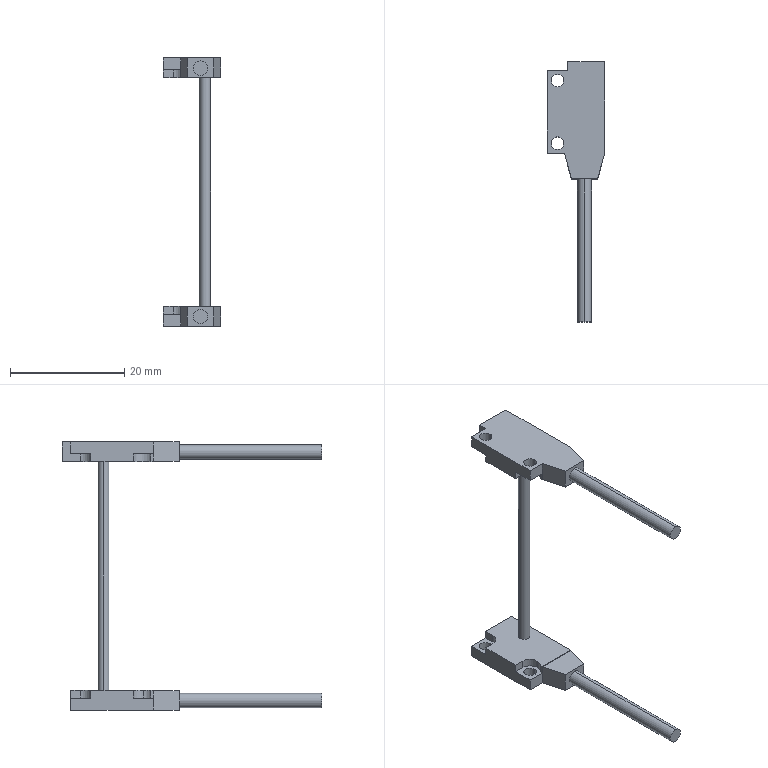Part | SolidWorks | features BaseBody 2, ICE 1 | 1 solid | 66 faces | box 10 x 45.5 x 47 mm | volume 1499 mm3 | plane 47 | cylinder 19 | commonest cylinder face diameters 2.2 x8 3.6 x5 2.5 x4 2 x2